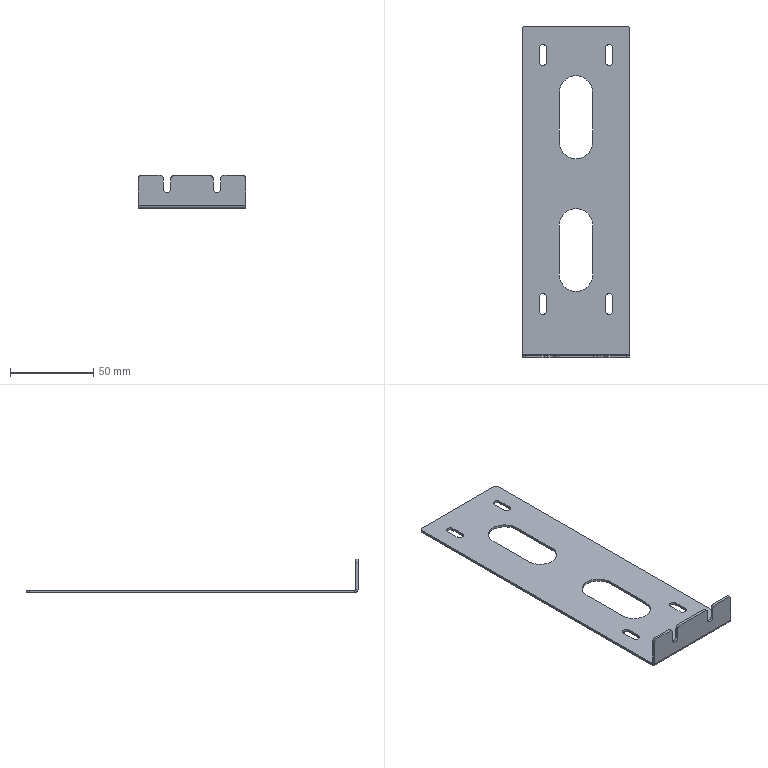Part | STEP file | Power supply mounting plate | 1 solid | 54 faces | box 65 x 200 x 20 mm | volume 18055 mm3 | plane 30 | cylinder 24 | commonest cylinder face diameters 4.5 x10 4 x9 20 x4 1 x1